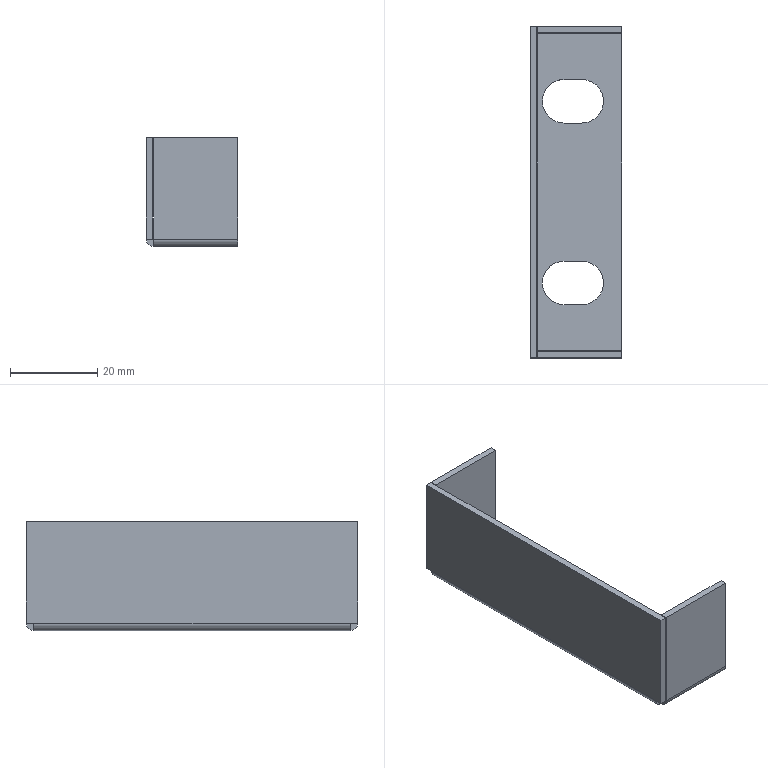Part | SolidWorks | features Cut 5, EdgeFlange 3, ICE 2, FlatPattern 1, MirrorPattern 1, SMBaseFlange 1, SheetMetal 1 | 1 solid | 42 faces | box 21 x 76 x 25 mm | volume 6000 mm3 | plane 30 | cylinder 12 | commonest cylinder face diameters 10 x6 0.4 x3 3.4 x3
STEP:
#1=CARTESIAN_POINT('',(-2.7,25.8,0.));
#2=VERTEX_POINT('',#1);
#3=CARTESIAN_POINT('',(-7.7,20.8,0.));
#4=VERTEX_POINT('',#3);
#5=CARTESIAN_POINT('',(-2.7,20.8,0.));
#6=DIRECTION('',(0.,0.,1.));
#7=DIRECTION('',(1.,0.,0.));
#8=AXIS2_PLACEMENT_3D('',#5,#6,#7);
#9=CIRCLE('',#8,5.);
#10=EDGE_CURVE('',#2,#4,#9,.T.);
#11=ORIENTED_EDGE('',*,*,#10,.T.);
#12=CARTESIAN_POINT('',(-7.7,20.8,-1.5));
#13=VERTEX_POINT('',#12);
#14=CARTESIAN_POINT('',(-7.7,20.8,8.5));
#15=DIRECTION('',(0.,0.,-1.));
#16=VECTOR('',#15,1000.);
#17=LINE('',#14,#16);
#18=EDGE_CURVE('',#4,#13,#17,.T.);
#19=ORIENTED_EDGE('',*,*,#18,.T.);
#20=CARTESIAN_POINT('',(-2.7,25.8,-1.5));
#21=VERTEX_POINT('',#20);
#22=CARTESIAN_POINT('',(-2.7,20.8,-1.5));
#23=DIRECTION('',(0.,0.,-1.));
#24=DIRECTION('',(-1.,0.,0.));
#25=AXIS2_PLACEMENT_3D('',#22,#23,#24);
#26=CIRCLE('',#25,5.);
#27=EDGE_CURVE('',#13,#21,#26,.T.);
#28=ORIENTED_EDGE('',*,*,#27,.T.);
#29=CARTESIAN_POINT('',(-2.7,25.8,8.5));
#30=DIRECTION('',(0.,0.,-1.));
#31=VECTOR('',#30,1000.);
#32=LINE('',#29,#31);
#33=EDGE_CURVE('',#2,#21,#32,.T.);
#34=ORIENTED_EDGE('',*,*,#33,.F.);
#35=EDGE_LOOP('',(#11,#19,#28,#34));
#36=FACE_OUTER_BOUND('',#35,.T.);
#37=CARTESIAN_POINT('',(-2.7,20.8,8.5));
#38=DIRECTION('',(0.,0.,-1.));
#39=DIRECTION('',(-1.,0.,0.));
#40=AXIS2_PLACEMENT_3D('',#37,#38,#39);
#41=CYLINDRICAL_SURFACE('',#40,5.);
#42=ADVANCED_FACE('',(#36),#41,.F.);
#43=CARTESIAN_POINT('',(-2.7,-15.8,0.));
#44=VERTEX_POINT('',#43);
#45=CARTESIAN_POINT('',(-7.7,-20.8,0.));
#46=VERTEX_POINT('',#45);
#47=CARTESIAN_POINT('',(-2.7,-20.8,0.));
#48=DIRECTION('',(0.,0.,1.));
#49=DIRECTION('',(1.,0.,0.));
#50=AXIS2_PLACEMENT_3D('',#47,#48,#49);
#51=CIRCLE('',#50,5.);
#52=EDGE_CURVE('',#44,#46,#51,.T.);
#53=ORIENTED_EDGE('',*,*,#52,.T.);
#54=CARTESIAN_POINT('',(-7.7,-20.8,-1.5));
#55=VERTEX_POINT('',#54);
#56=CARTESIAN_POINT('',(-7.7,-20.8,8.5));
#57=DIRECTION('',(0.,0.,-1.));
#58=VECTOR('',#57,1000.);
#59=LINE('',#56,#58);
#60=EDGE_CURVE('',#46,#55,#59,.T.);
#61=ORIENTED_EDGE('',*,*,#60,.T.);
#62=CARTESIAN_POINT('',(-2.7,-15.8,-1.5));
#63=VERTEX_POINT('',#62);
#64=CARTESIAN_POINT('',(-2.7,-20.8,-1.5));
#65=DIRECTION('',(0.,0.,-1.));
#66=DIRECTION('',(1.,0.,0.));
#67=AXIS2_PLACEMENT_3D('',#64,#65,#66);
#68=CIRCLE('',#67,5.);
#69=EDGE_CURVE('',#55,#63,#68,.T.);
#70=ORIENTED_EDGE('',*,*,#69,.T.);
#71=CARTESIAN_POINT('',(-2.7,-15.8,8.5));
#72=DIRECTION('',(0.,0.,-1.));
#73=VECTOR('',#72,1000.);
#74=LINE('',#71,#73);
#75=EDGE_CURVE('',#44,#63,#74,.T.);
#76=ORIENTED_EDGE('',*,*,#75,.F.);
#77=EDGE_LOOP('',(#53,#61,#70,#76));
#78=FACE_OUTER_BOUND('',#77,.T.);
#79=CARTESIAN_POINT('',(-2.7,-20.8,8.5));
#80=DIRECTION('',(0.,0.,-1.));
#81=DIRECTION('',(-1.,0.,0.));
#82=AXIS2_PLACEMENT_3D('',#79,#80,#81);
#83=CYLINDRICAL_SURFACE('',#82,5.);
#84=ADVANCED_FACE('',(#78),#83,.F.);
#85=CARTESIAN_POINT('',(-9.,-36.3,0.2));
#86=VERTEX_POINT('',#85);
#87=CARTESIAN_POINT('',(-10.5,-36.3,0.2));
#88=VERTEX_POINT('',#87);
#89=CARTESIAN_POINT('',(-9.,-36.3,0.2));
#90=DIRECTION('',(-1.,0.,0.));
#91=VECTOR('',#90,1000.);
#92=LINE('',#89,#91);
#93=EDGE_CURVE('',#86,#88,#92,.T.);
#94=ORIENTED_EDGE('',*,*,#93,.F.);
#95=CARTESIAN_POINT('',(-9.,-38.,0.2));
#96=VERTEX_POINT('',#95);
#97=CARTESIAN_POINT('',(-9.,38.,0.2));
#98=DIRECTION('',(0.,-1.,0.));
#99=VECTOR('',#98,1000.);
#100=LINE('',#97,#99);
#101=EDGE_CURVE('',#86,#96,#100,.T.);
#102=ORIENTED_EDGE('',*,*,#101,.T.);
#103=CARTESIAN_POINT('',(-10.5,-38.,0.2));
#104=VERTEX_POINT('',#103);
#105=CARTESIAN_POINT('',(-9.,-38.,0.2));
#106=DIRECTION('',(-1.,0.,0.));
#107=VECTOR('',#106,1000.);
#108=LINE('',#105,#107);
#109=EDGE_CURVE('',#96,#104,#108,.T.);
#110=ORIENTED_EDGE('',*,*,#109,.T.);
#111=CARTESIAN_POINT('',(-10.5,38.,0.2));
#112=DIRECTION('',(0.,1.,0.));
#113=VECTOR('',#112,1000.);
#114=LINE('',#111,#113);
#115=EDGE_CURVE('',#104,#88,#114,.T.);
#116=ORIENTED_EDGE('',*,*,#115,.T.);
#117=EDGE_LOOP('',(#94,#102,#110,#116));
#118=FACE_OUTER_BOUND('',#117,.T.);
#119=CARTESIAN_POINT('',(0.,0.,0.2));
#120=DIRECTION('',(0.,0.,1.));
#121=DIRECTION('',(1.,0.,0.));
#122=AXIS2_PLACEMENT_3D('',#119,#120,#121);
#123=PLANE('',#122);
#124=ADVANCED_FACE('',(#118),#123,.F.);
#125=CARTESIAN_POINT('',(-8.8,-36.3,-1.5));
#126=VERTEX_POINT('',#125);
#127=CARTESIAN_POINT('',(-8.8,36.3,-1.5));
#128=VERTEX_POINT('',#127);
#129=CARTESIAN_POINT('',(-8.8,-38.,-1.5));
#130=DIRECTION('',(0.,1.,0.));
#131=VECTOR('',#130,1000.);
#132=LINE('',#129,#131);
#133=EDGE_CURVE('',#126,#128,#132,.T.);
#134=ORIENTED_EDGE('',*,*,#133,.F.);
#135=CARTESIAN_POINT('',(-8.8,-36.3,0.2));
#136=DIRECTION('',(0.,1.,0.));
#137=DIRECTION('',(0.,0.,-1.));
#138=AXIS2_PLACEMENT_3D('',#135,#136,#137);
#139=CIRCLE('',#138,1.7);
#140=EDGE_CURVE('',#126,#88,#139,.T.);
#141=ORIENTED_EDGE('',*,*,#140,.T.);
#142=CARTESIAN_POINT('',(-10.5,36.3,0.2));
#143=VERTEX_POINT('',#142);
#144=CARTESIAN_POINT('',(-10.5,38.,0.2));
#145=DIRECTION('',(0.,1.,0.));
#146=VECTOR('',#145,1000.);
#147=LINE('',#144,#146);
#148=EDGE_CURVE('',#88,#143,#147,.T.);
#149=ORIENTED_EDGE('',*,*,#148,.T.);
#150=CARTESIAN_POINT('',(-8.8,36.3,0.2));
#151=DIRECTION('',(0.,-1.,0.));
#152=DIRECTION('',(0.,0.,1.));
#153=AXIS2_PLACEMENT_3D('',#150,#151,#152);
#154=CIRCLE('',#153,1.7);
#155=EDGE_CURVE('',#143,#128,#154,.T.);
#156=ORIENTED_EDGE('',*,*,#155,.T.);
#157=EDGE_LOOP('',(#134,#141,#149,#156));
#158=FACE_OUTER_BOUND('',#157,.T.);
#159=CARTESIAN_POINT('',(-8.8,-38.,0.2));
#160=DIRECTION('',(0.,-1.,0.));
#161=DIRECTION('',(-1.,0.,0.));
#162=AXIS2_PLACEMENT_3D('',#159,#160,#161);
#163=CYLINDRICAL_SURFACE('',#162,1.7);
#164=ADVANCED_FACE('',(#158),#163,.T.);
#165=CARTESIAN_POINT('',(-8.8,-36.3,0.));
#166=VERTEX_POINT('',#165);
#167=CARTESIAN_POINT('',(-8.8,-36.3,0.2));
#168=DIRECTION('',(0.,1.,0.));
#169=DIRECTION('',(0.,0.,-1.));
#170=AXIS2_PLACEMENT_3D('',#167,#168,#169);
#171=CIRCLE('',#170,0.2);
#172=EDGE_CURVE('',#166,#86,#171,.T.);
#173=ORIENTED_EDGE('',*,*,#172,.T.);
#174=ORIENTED_EDGE('',*,*,#93,.T.);
#175=ORIENTED_EDGE('',*,*,#140,.F.);
#176=CARTESIAN_POINT('',(-8.8,-36.3,0.));
#177=DIRECTION('',(0.,0.,-1.));
#178=VECTOR('',#177,1000.);
#179=LINE('',#176,#178);
#180=EDGE_CURVE('',#166,#126,#179,.T.);
#181=ORIENTED_EDGE('',*,*,#180,.F.);
#182=EDGE_LOOP('',(#173,#174,#175,#181));
#183=FACE_OUTER_BOUND('',#182,.T.);
#184=CARTESIAN_POINT('',(-8.8,-36.3,0.2));
#185=DIRECTION('',(0.,-1.,0.));
#186=DIRECTION('',(0.,0.,-1.));
#187=AXIS2_PLACEMENT_3D('',#184,#185,#186);
#188=PLANE('',#187);
#189=ADVANCED_FACE('',(#183),#188,.T.);
#190=CARTESIAN_POINT('',(1.3,15.8,-1.5));
#191=VERTEX_POINT('',#190);
#192=CARTESIAN_POINT('',(-2.7,15.8,-1.5));
#193=VERTEX_POINT('',#192);
#194=CARTESIAN_POINT('',(1.3,15.8,-1.5));
#195=DIRECTION('',(-1.,0.,0.));
#196=VECTOR('',#195,1000.);
#197=LINE('',#194,#196);
#198=EDGE_CURVE('',#191,#193,#197,.T.);
#199=ORIENTED_EDGE('',*,*,#198,.F.);
#200=CARTESIAN_POINT('',(1.3,25.8,-1.5));
#201=VERTEX_POINT('',#200);
#202=CARTESIAN_POINT('',(1.3,20.8,-1.5));
#203=DIRECTION('',(0.,0.,-1.));
#204=DIRECTION('',(-1.,0.,0.));
#205=AXIS2_PLACEMENT_3D('',#202,#203,#204);
#206=CIRCLE('',#205,5.);
#207=EDGE_CURVE('',#201,#191,#206,.T.);
#208=ORIENTED_EDGE('',*,*,#207,.F.);
#209=CARTESIAN_POINT('',(1.3,25.8,-1.5));
#210=DIRECTION('',(1.,0.,0.));
#211=VECTOR('',#210,1000.);
#212=LINE('',#209,#211);
#213=EDGE_CURVE('',#21,#201,#212,.T.);
#214=ORIENTED_EDGE('',*,*,#213,.F.);
#215=ORIENTED_EDGE('',*,*,#27,.F.);
#216=CARTESIAN_POINT('',(-2.7,20.8,-1.5));
#217=DIRECTION('',(0.,0.,-1.));
#218=DIRECTION('',(-1.,0.,0.));
#219=AXIS2_PLACEMENT_3D('',#216,#217,#218);
#220=CIRCLE('',#219,5.);
#221=EDGE_CURVE('',#193,#13,#220,.T.);
#222=ORIENTED_EDGE('',*,*,#221,.F.);
#223=EDGE_LOOP('',(#199,#208,#214,#215,#222));
#224=FACE_BOUND('',#223,.T.);
#225=CARTESIAN_POINT('',(1.3,-25.8,-1.5));
#226=VERTEX_POINT('',#225);
#227=CARTESIAN_POINT('',(-2.7,-25.8,-1.5));
#228=VERTEX_POINT('',#227);
#229=CARTESIAN_POINT('',(1.3,-25.8,-1.5));
#230=DIRECTION('',(-1.,0.,0.));
#231=VECTOR('',#230,1000.);
#232=LINE('',#229,#231);
#233=EDGE_CURVE('',#226,#228,#232,.T.);
#234=ORIENTED_EDGE('',*,*,#233,.F.);
#235=CARTESIAN_POINT('',(1.3,-15.8,-1.5));
#236=VERTEX_POINT('',#235);
#237=CARTESIAN_POINT('',(1.3,-20.8,-1.5));
#238=DIRECTION('',(0.,0.,-1.));
#239=DIRECTION('',(1.,0.,0.));
#240=AXIS2_PLACEMENT_3D('',#237,#238,#239);
#241=CIRCLE('',#240,5.);
#242=EDGE_CURVE('',#236,#226,#241,.T.);
#243=ORIENTED_EDGE('',*,*,#242,.F.);
#244=CARTESIAN_POINT('',(1.3,-15.8,-1.5));
#245=DIRECTION('',(1.,0.,0.));
#246=VECTOR('',#245,1000.);
#247=LINE('',#244,#246);
#248=EDGE_CURVE('',#63,#236,#247,.T.);
#249=ORIENTED_EDGE('',*,*,#248,.F.);
#250=ORIENTED_EDGE('',*,*,#69,.F.);
#251=CARTESIAN_POINT('',(-2.7,-20.8,-1.5));
#252=DIRECTION('',(0.,0.,-1.));
#253=DIRECTION('',(1.,0.,0.));
#254=AXIS2_PLACEMENT_3D('',#251,#252,#253);
#255=CIRCLE('',#254,5.);
#256=EDGE_CURVE('',#228,#55,#255,.T.);
#257=ORIENTED_EDGE('',*,*,#256,.F.);
#258=EDGE_LOOP('',(#234,#243,#249,#250,#257));
#259=FACE_BOUND('',#258,.T.);
#260=CARTESIAN_POINT('',(10.5,-36.3,-1.5));
#261=VERTEX_POINT('',#260);
#262=CARTESIAN_POINT('',(10.5,-36.3,-1.5));
#263=DIRECTION('',(-1.,0.,0.));
#264=VECTOR('',#263,1000.);
#265=LINE('',#262,#264);
#266=EDGE_CURVE('',#261,#126,#265,.T.);
#267=ORIENTED_EDGE('',*,*,#266,.T.);
#268=ORIENTED_EDGE('',*,*,#133,.T.);
#269=CARTESIAN_POINT('',(10.5,36.3,-1.5));
#270=VERTEX_POINT('',#269);
#271=CARTESIAN_POINT('',(-8.8,36.3,-1.5));
#272=DIRECTION('',(1.,0.,0.));
#273=VECTOR('',#272,1000.);
#274=LINE('',#271,#273);
#275=EDGE_CURVE('',#128,#270,#274,.T.);
#276=ORIENTED_EDGE('',*,*,#275,.T.);
#277=CARTESIAN_POINT('',(10.5,38.,-1.5));
#278=DIRECTION('',(0.,1.,0.));
#279=VECTOR('',#278,1000.);
#280=LINE('',#277,#279);
#281=EDGE_CURVE('',#261,#270,#280,.T.);
#282=ORIENTED_EDGE('',*,*,#281,.F.);
#283=EDGE_LOOP('',(#267,#268,#276,#282));
#284=FACE_OUTER_BOUND('',#283,.T.);
#285=CARTESIAN_POINT('',(0.,0.,-1.5));
#286=DIRECTION('',(0.,0.,1.));
#287=DIRECTION('',(1.,0.,0.));
#288=AXIS2_PLACEMENT_3D('',#285,#286,#287);
#289=PLANE('',#288);
#290=ADVANCED_FACE('',(#224,#259,#284),#289,.F.);
#291=CARTESIAN_POINT('',(1.3,15.8,0.));
#292=VERTEX_POINT('',#291);
#293=CARTESIAN_POINT('',(1.3,25.8,0.));
#294=VERTEX_POINT('',#293);
#295=CARTESIAN_POINT('',(1.3,20.8,0.));
#296=DIRECTION('',(0.,0.,1.));
#297=DIRECTION('',(1.,0.,0.));
#298=AXIS2_PLACEMENT_3D('',#295,#296,#297);
#299=CIRCLE('',#298,5.);
#300=EDGE_CURVE('',#292,#294,#299,.T.);
#301=ORIENTED_EDGE('',*,*,#300,.F.);
#302=CARTESIAN_POINT('',(-2.7,15.8,0.));
#303=VERTEX_POINT('',#302);
#304=CARTESIAN_POINT('',(0.,15.8,0.));
#305=DIRECTION('',(1.,0.,0.));
#306=VECTOR('',#305,1000.);
#307=LINE('',#304,#306);
#308=EDGE_CURVE('',#303,#292,#307,.T.);
#309=ORIENTED_EDGE('',*,*,#308,.F.);
#310=CARTESIAN_POINT('',(-2.7,20.8,0.));
#311=DIRECTION('',(0.,0.,1.));
#312=DIRECTION('',(1.,0.,0.));
#313=AXIS2_PLACEMENT_3D('',#310,#311,#312);
#314=CIRCLE('',#313,5.);
#315=EDGE_CURVE('',#4,#303,#314,.T.);
#316=ORIENTED_EDGE('',*,*,#315,.F.);
#317=ORIENTED_EDGE('',*,*,#10,.F.);
#318=CARTESIAN_POINT('',(0.,25.8,0.));
#319=DIRECTION('',(-1.,0.,0.));
#320=VECTOR('',#319,1000.);
#321=LINE('',#318,#320);
#322=EDGE_CURVE('',#294,#2,#321,.T.);
#323=ORIENTED_EDGE('',*,*,#322,.F.);
#324=EDGE_LOOP('',(#301,#309,#316,#317,#323));
#325=FACE_BOUND('',#324,.T.);
#326=CARTESIAN_POINT('',(1.3,-25.8,0.));
#327=VERTEX_POINT('',#326);
#328=CARTESIAN_POINT('',(1.3,-15.8,0.));
#329=VERTEX_POINT('',#328);
#330=CARTESIAN_POINT('',(1.3,-20.8,0.));
#331=DIRECTION('',(0.,0.,1.));
#332=DIRECTION('',(1.,0.,0.));
#333=AXIS2_PLACEMENT_3D('',#330,#331,#332);
#334=CIRCLE('',#333,5.);
#335=EDGE_CURVE('',#327,#329,#334,.T.);
#336=ORIENTED_EDGE('',*,*,#335,.F.);
#337=CARTESIAN_POINT('',(-2.7,-25.8,0.));
#338=VERTEX_POINT('',#337);
#339=CARTESIAN_POINT('',(0.,-25.8,0.));
#340=DIRECTION('',(1.,0.,0.));
#341=VECTOR('',#340,1000.);
#342=LINE('',#339,#341);
#343=EDGE_CURVE('',#338,#327,#342,.T.);
#344=ORIENTED_EDGE('',*,*,#343,.F.);
#345=CARTESIAN_POINT('',(-2.7,-20.8,0.));
#346=DIRECTION('',(0.,0.,1.));
#347=DIRECTION('',(1.,0.,0.));
#348=AXIS2_PLACEMENT_3D('',#345,#346,#347);
#349=CIRCLE('',#348,5.);
#350=EDGE_CURVE('',#46,#338,#349,.T.);
#351=ORIENTED_EDGE('',*,*,#350,.F.);
#352=ORIENTED_EDGE('',*,*,#52,.F.);
#353=CARTESIAN_POINT('',(0.,-15.8,0.));
#354=DIRECTION('',(-1.,0.,0.));
#355=VECTOR('',#354,1000.);
#356=LINE('',#353,#355);
#357=EDGE_CURVE('',#329,#44,#356,.T.);
#358=ORIENTED_EDGE('',*,*,#357,.F.);
#359=EDGE_LOOP('',(#336,#344,#351,#352,#358));
#360=FACE_BOUND('',#359,.T.);
#361=CARTESIAN_POINT('',(-8.8,36.3,0.));
#362=VERTEX_POINT('',#361);
#363=CARTESIAN_POINT('',(-8.8,-38.,0.));
#364=DIRECTION('',(0.,1.,0.));
#365=VECTOR('',#364,1000.);
#366=LINE('',#363,#365);
#367=EDGE_CURVE('',#166,#362,#366,.T.);
#368=ORIENTED_EDGE('',*,*,#367,.F.);
#369=CARTESIAN_POINT('',(10.5,-36.3,0.));
#370=VERTEX_POINT('',#369);
#371=CARTESIAN_POINT('',(10.5,-36.3,0.));
#372=DIRECTION('',(-1.,0.,0.));
#373=VECTOR('',#372,1000.);
#374=LINE('',#371,#373);
#375=EDGE_CURVE('',#370,#166,#374,.T.);
#376=ORIENTED_EDGE('',*,*,#375,.F.);
#377=CARTESIAN_POINT('',(10.5,36.3,0.));
#378=VERTEX_POINT('',#377);
#379=CARTESIAN_POINT('',(10.5,38.,0.));
#380=DIRECTION('',(0.,1.,0.));
#381=VECTOR('',#380,1000.);
#382=LINE('',#379,#381);
#383=EDGE_CURVE('',#370,#378,#382,.T.);
#384=ORIENTED_EDGE('',*,*,#383,.T.);
#385=CARTESIAN_POINT('',(-8.8,36.3,0.));
#386=DIRECTION('',(1.,0.,0.));
#387=VECTOR('',#386,1000.);
#388=LINE('',#385,#387);
#389=EDGE_CURVE('',#362,#378,#388,.T.);
#390=ORIENTED_EDGE('',*,*,#389,.F.);
#391=EDGE_LOOP('',(#368,#376,#384,#390));
#392=FACE_OUTER_BOUND('',#391,.T.);
#393=CARTESIAN_POINT('',(0.,0.,0.));
#394=DIRECTION('',(0.,0.,1.));
#395=DIRECTION('',(1.,0.,0.));
#396=AXIS2_PLACEMENT_3D('',#393,#394,#395);
#397=PLANE('',#396);
#398=ADVANCED_FACE('',(#325,#360,#392),#397,.T.);
#399=ORIENTED_EDGE('',*,*,#383,.F.);
#400=CARTESIAN_POINT('',(10.5,-36.3,0.));
#401=DIRECTION('',(0.,0.,-1.));
#402=VECTOR('',#401,1000.);
#403=LINE('',#400,#402);
#404=EDGE_CURVE('',#370,#261,#403,.T.);
#405=ORIENTED_EDGE('',*,*,#404,.T.);
#406=ORIENTED_EDGE('',*,*,#281,.T.);
#407=CARTESIAN_POINT('',(10.5,36.3,0.));
#408=DIRECTION('',(0.,0.,-1.));
#409=VECTOR('',#408,1000.);
#410=LINE('',#407,#409);
#411=EDGE_CURVE('',#378,#270,#410,.T.);
#412=ORIENTED_EDGE('',*,*,#411,.F.);
#413=EDGE_LOOP('',(#399,#405,#406,#412));
#414=FACE_OUTER_BOUND('',#413,.T.);
#415=CARTESIAN_POINT('',(10.5,38.,-1.5));
#416=DIRECTION('',(1.,0.,0.));
#417=DIRECTION('',(0.,0.,-1.));
#418=AXIS2_PLACEMENT_3D('',#415,#416,#417);
#419=PLANE('',#418);
#420=ADVANCED_FACE('',(#414),#419,.T.);
#421=CARTESIAN_POINT('',(-9.,36.3,0.2));
#422=VERTEX_POINT('',#421);
#423=CARTESIAN_POINT('',(-10.5,36.3,0.2));
#424=DIRECTION('',(1.,0.,0.));
#425=VECTOR('',#424,1000.);
#426=LINE('',#423,#425);
#427=EDGE_CURVE('',#143,#422,#426,.T.);
#428=ORIENTED_EDGE('',*,*,#427,.F.);
#429=CARTESIAN_POINT('',(-10.5,38.,0.2));
#430=VERTEX_POINT('',#429);
#431=CARTESIAN_POINT('',(-10.5,38.,0.2));
#432=DIRECTION('',(0.,1.,0.));
#433=VECTOR('',#432,1000.);
#434=LINE('',#431,#433);
#435=EDGE_CURVE('',#143,#430,#434,.T.);
#436=ORIENTED_EDGE('',*,*,#435,.T.);
#437=CARTESIAN_POINT('',(-9.,38.,0.2));
#438=VERTEX_POINT('',#437);
#439=CARTESIAN_POINT('',(-10.5,38.,0.2));
#440=DIRECTION('',(-1.,0.,0.));
#441=VECTOR('',#440,1000.);
#442=LINE('',#439,#441);
#443=EDGE_CURVE('',#438,#430,#442,.T.);
#444=ORIENTED_EDGE('',*,*,#443,.F.);
#445=CARTESIAN_POINT('',(-9.,38.,0.2));
#446=DIRECTION('',(0.,-1.,0.));
#447=VECTOR('',#446,1000.);
#448=LINE('',#445,#447);
#449=EDGE_CURVE('',#438,#422,#448,.T.);
#450=ORIENTED_EDGE('',*,*,#449,.T.);
#451=EDGE_LOOP('',(#428,#436,#444,#450));
#452=FACE_OUTER_BOUND('',#451,.T.);
#453=CARTESIAN_POINT('',(0.,0.,0.2));
#454=DIRECTION('',(0.,0.,-1.));
#455=DIRECTION('',(-1.,0.,0.));
#456=AXIS2_PLACEMENT_3D('',#453,#454,#455);
#457=PLANE('',#456);
#458=ADVANCED_FACE('',(#452),#457,.T.);
#459=ORIENTED_EDGE('',*,*,#155,.F.);
#460=ORIENTED_EDGE('',*,*,#427,.T.);
#461=CARTESIAN_POINT('',(-8.8,36.3,0.2));
#462=DIRECTION('',(0.,-1.,0.));
#463=DIRECTION('',(0.,0.,1.));
#464=AXIS2_PLACEMENT_3D('',#461,#462,#463);
#465=CIRCLE('',#464,0.2);
#466=EDGE_CURVE('',#422,#362,#465,.T.);
#467=ORIENTED_EDGE('',*,*,#466,.T.);
#468=CARTESIAN_POINT('',(-8.8,36.3,0.));
#469=DIRECTION('',(0.,0.,-1.));
#470=VECTOR('',#469,1000.);
#471=LINE('',#468,#470);
#472=EDGE_CURVE('',#362,#128,#471,.T.);
#473=ORIENTED_EDGE('',*,*,#472,.T.);
#474=EDGE_LOOP('',(#459,#460,#467,#473));
#475=FACE_OUTER_BOUND('',#474,.T.);
#476=CARTESIAN_POINT('',(-8.8,36.3,0.2));
#477=DIRECTION('',(0.,1.,0.));
#478=DIRECTION('',(0.,0.,1.));
#479=AXIS2_PLACEMENT_3D('',#476,#477,#478);
#480=PLANE('',#479);
#481=ADVANCED_FACE('',(#475),#480,.T.);
#482=ORIENTED_EDGE('',*,*,#172,.F.);
#483=ORIENTED_EDGE('',*,*,#367,.T.);
#484=ORIENTED_EDGE('',*,*,#466,.F.);
#485=CARTESIAN_POINT('',(-9.,38.,0.2));
#486=DIRECTION('',(0.,-1.,0.));
#487=VECTOR('',#486,1000.);
#488=LINE('',#485,#487);
#489=EDGE_CURVE('',#422,#86,#488,.T.);
#490=ORIENTED_EDGE('',*,*,#489,.T.);
#491=EDGE_LOOP('',(#482,#483,#484,#490));
#492=FACE_OUTER_BOUND('',#491,.T.);
#493=CARTESIAN_POINT('',(-8.8,-38.,0.2));
#494=DIRECTION('',(0.,-1.,0.));
#495=DIRECTION('',(-1.,0.,0.));
#496=AXIS2_PLACEMENT_3D('',#493,#494,#495);
#497=CYLINDRICAL_SURFACE('',#496,0.2);
#498=ADVANCED_FACE('',(#492),#497,.F.);
#499=ORIENTED_EDGE('',*,*,#443,.T.);
#500=CARTESIAN_POINT('',(-10.5,38.,23.5));
#501=VERTEX_POINT('',#500);
#502=CARTESIAN_POINT('',(-10.5,38.,0.));
#503=DIRECTION('',(0.,0.,-1.));
#504=VECTOR('',#503,1000.);
#505=LINE('',#502,#504);
#506=EDGE_CURVE('',#501,#430,#505,.T.);
#507=ORIENTED_EDGE('',*,*,#506,.F.);
#508=CARTESIAN_POINT('',(-9.,38.,23.5));
#509=VERTEX_POINT('',#508);
#510=CARTESIAN_POINT('',(-10.5,38.,23.5));
#511=DIRECTION('',(1.,0.,0.));
#512=VECTOR('',#511,1000.);
#513=LINE('',#510,#512);
#514=EDGE_CURVE('',#501,#509,#513,.T.);
#515=ORIENTED_EDGE('',*,*,#514,.T.);
#516=CARTESIAN_POINT('',(-9.,38.,0.));
#517=DIRECTION('',(0.,0.,-1.));
#518=VECTOR('',#517,1000.);
#519=LINE('',#516,#518);
#520=EDGE_CURVE('',#509,#438,#519,.T.);
#521=ORIENTED_EDGE('',*,*,#520,.T.);
#522=EDGE_LOOP('',(#499,#507,#515,#521));
#523=FACE_OUTER_BOUND('',#522,.T.);
#524=CARTESIAN_POINT('',(-10.5,38.,0.));
#525=DIRECTION('',(0.,-1.,0.));
#526=DIRECTION('',(0.,0.,-1.));
#527=AXIS2_PLACEMENT_3D('',#524,#525,#526);
#528=PLANE('',#527);
#529=ADVANCED_FACE('',(#523),#528,.F.);
#530=ORIENTED_EDGE('',*,*,#109,.F.);
#531=CARTESIAN_POINT('',(-9.,-38.,23.5));
#532=VERTEX_POINT('',#531);
#533=CARTESIAN_POINT('',(-9.,-38.,23.5));
#534=DIRECTION('',(0.,0.,1.));
#535=VECTOR('',#534,1000.);
#536=LINE('',#533,#535);
#537=EDGE_CURVE('',#96,#532,#536,.T.);
#538=ORIENTED_EDGE('',*,*,#537,.T.);
#539=CARTESIAN_POINT('',(-10.5,-38.,23.5));
#540=VERTEX_POINT('',#539);
#541=CARTESIAN_POINT('',(-10.5,-38.,23.5));
#542=DIRECTION('',(1.,0.,0.));
#543=VECTOR('',#542,1000.);
#544=LINE('',#541,#543);
#545=EDGE_CURVE('',#540,#532,#544,.T.);
#546=ORIENTED_EDGE('',*,*,#545,.F.);
#547=CARTESIAN_POINT('',(-10.5,-38.,0.));
#548=DIRECTION('',(0.,0.,1.));
#549=VECTOR('',#548,1000.);
#550=LINE('',#547,#549);
#551=EDGE_CURVE('',#104,#540,#550,.T.);
#552=ORIENTED_EDGE('',*,*,#551,.F.);
#553=EDGE_LOOP('',(#530,#538,#546,#552));
#554=FACE_OUTER_BOUND('',#553,.T.);
#555=CARTESIAN_POINT('',(-10.5,-38.,23.5));
#556=DIRECTION('',(0.,1.,0.));
#557=DIRECTION('',(0.,0.,1.));
#558=AXIS2_PLACEMENT_3D('',#555,#556,#557);
#559=PLANE('',#558);
#560=ADVANCED_FACE('',(#554),#559,.F.);
#561=ORIENTED_EDGE('',*,*,#115,.F.);
#562=ORIENTED_EDGE('',*,*,#551,.T.);
#563=CARTESIAN_POINT('',(-10.5,0.,23.5));
#564=DIRECTION('',(0.,1.,0.));
#565=VECTOR('',#564,1000.);
#566=LINE('',#563,#565);
#567=EDGE_CURVE('',#540,#501,#566,.T.);
#568=ORIENTED_EDGE('',*,*,#567,.T.);
#569=ORIENTED_EDGE('',*,*,#506,.T.);
#570=ORIENTED_EDGE('',*,*,#435,.F.);
#571=ORIENTED_EDGE('',*,*,#148,.F.);
#572=EDGE_LOOP('',(#561,#562,#568,#569,#570,#571));
#573=FACE_OUTER_BOUND('',#572,.T.);
#574=CARTESIAN_POINT('',(-10.5,0.,0.));
#575=DIRECTION('',(1.,0.,0.));
#576=DIRECTION('',(0.,0.,-1.));
#577=AXIS2_PLACEMENT_3D('',#574,#575,#576);
#578=PLANE('',#577);
#579=ADVANCED_FACE('',(#573),#578,.F.);
#580=ORIENTED_EDGE('',*,*,#537,.F.);
#581=ORIENTED_EDGE('',*,*,#101,.F.);
#582=ORIENTED_EDGE('',*,*,#489,.F.);
#583=ORIENTED_EDGE('',*,*,#449,.F.);
#584=ORIENTED_EDGE('',*,*,#520,.F.);
#585=CARTESIAN_POINT('',(-9.,38.,23.5));
#586=DIRECTION('',(0.,1.,0.));
#587=VECTOR('',#586,1000.);
#588=LINE('',#585,#587);
#589=EDGE_CURVE('',#532,#509,#588,.T.);
#590=ORIENTED_EDGE('',*,*,#589,.F.);
#591=EDGE_LOOP('',(#580,#581,#582,#583,#584,#590));
#592=FACE_OUTER_BOUND('',#591,.T.);
#593=CARTESIAN_POINT('',(-9.,0.,0.));
#594=DIRECTION('',(1.,0.,0.));
#595=DIRECTION('',(0.,0.,-1.));
#596=AXIS2_PLACEMENT_3D('',#593,#594,#595);
#597=PLANE('',#596);
#598=ADVANCED_FACE('',(#592),#597,.T.);
#599=ORIENTED_EDGE('',*,*,#589,.T.);
#600=ORIENTED_EDGE('',*,*,#514,.F.);
#601=ORIENTED_EDGE('',*,*,#567,.F.);
#602=ORIENTED_EDGE('',*,*,#545,.T.);
#603=EDGE_LOOP('',(#599,#600,#601,#602));
#604=FACE_OUTER_BOUND('',#603,.T.);
#605=CARTESIAN_POINT('',(-10.5,38.,23.5));
#606=DIRECTION('',(0.,0.,-1.));
#607=DIRECTION('',(-1.,0.,0.));
#608=AXIS2_PLACEMENT_3D('',#605,#606,#607);
#609=PLANE('',#608);
#610=ADVANCED_FACE('',(#604),#609,.F.);
#611=CARTESIAN_POINT('',(10.5,36.5,0.2));
#612=VERTEX_POINT('',#611);
#613=CARTESIAN_POINT('',(10.5,38.,0.2));
#614=VERTEX_POINT('',#613);
#615=CARTESIAN_POINT('',(10.5,38.,0.2));
#616=DIRECTION('',(0.,1.,0.));
#617=VECTOR('',#616,1000.);
#618=LINE('',#615,#617);
#619=EDGE_CURVE('',#612,#614,#618,.T.);
#620=ORIENTED_EDGE('',*,*,#619,.F.);
#621=CARTESIAN_POINT('',(10.5,36.3,0.2));
#622=DIRECTION('',(1.,0.,0.));
#623=DIRECTION('',(0.,0.,1.));
#624=AXIS2_PLACEMENT_3D('',#621,#622,#623);
#625=CIRCLE('',#624,0.2);
#626=EDGE_CURVE('',#378,#612,#625,.T.);
#627=ORIENTED_EDGE('',*,*,#626,.F.);
#628=ORIENTED_EDGE('',*,*,#411,.T.);
#629=CARTESIAN_POINT('',(10.5,36.3,0.2));
#630=DIRECTION('',(1.,0.,0.));
#631=DIRECTION('',(0.,0.,1.));
#632=AXIS2_PLACEMENT_3D('',#629,#630,#631);
#633=CIRCLE('',#632,1.7);
#634=EDGE_CURVE('',#270,#614,#633,.T.);
#635=ORIENTED_EDGE('',*,*,#634,.T.);
#636=EDGE_LOOP('',(#620,#627,#628,#635));
#637=FACE_OUTER_BOUND('',#636,.T.);
#638=CARTESIAN_POINT('',(10.5,36.3,0.2));
#639=DIRECTION('',(1.,0.,0.));
#640=DIRECTION('',(0.,0.,-1.));
#641=AXIS2_PLACEMENT_3D('',#638,#639,#640);
#642=PLANE('',#641);
#643=ADVANCED_FACE('',(#637),#642,.T.);
#644=CARTESIAN_POINT('',(-8.8,36.5,0.2));
#645=VERTEX_POINT('',#644);
#646=CARTESIAN_POINT('',(-8.8,36.3,0.2));
#647=DIRECTION('',(-1.,0.,0.));
#648=DIRECTION('',(0.,0.,1.));
#649=AXIS2_PLACEMENT_3D('',#646,#647,#648);
#650=CIRCLE('',#649,0.2);
#651=EDGE_CURVE('',#645,#362,#650,.T.);
#652=ORIENTED_EDGE('',*,*,#651,.F.);
#653=CARTESIAN_POINT('',(-8.8,38.,0.2));
#654=VERTEX_POINT('',#653);
#655=CARTESIAN_POINT('',(-8.8,36.5,0.2));
#656=DIRECTION('',(0.,1.,0.));
#657=VECTOR('',#656,1000.);
#658=LINE('',#655,#657);
#659=EDGE_CURVE('',#645,#654,#658,.T.);
#660=ORIENTED_EDGE('',*,*,#659,.T.);
#661=CARTESIAN_POINT('',(-8.8,36.3,0.2));
#662=DIRECTION('',(-1.,0.,0.));
#663=DIRECTION('',(0.,0.,1.));
#664=AXIS2_PLACEMENT_3D('',#661,#662,#663);
#665=CIRCLE('',#664,1.7);
#666=EDGE_CURVE('',#654,#128,#665,.T.);
#667=ORIENTED_EDGE('',*,*,#666,.T.);
#668=ORIENTED_EDGE('',*,*,#472,.F.);
#669=EDGE_LOOP('',(#652,#660,#667,#668));
#670=FACE_OUTER_BOUND('',#669,.T.);
#671=CARTESIAN_POINT('',(-8.8,36.3,0.2));
#672=DIRECTION('',(1.,0.,0.));
#673=DIRECTION('',(0.,0.,-1.));
#674=AXIS2_PLACEMENT_3D('',#671,#672,#673);
#675=PLANE('',#674);
#676=ADVANCED_FACE('',(#670),#675,.F.);
#677=ORIENTED_EDGE('',*,*,#275,.F.);
#678=ORIENTED_EDGE('',*,*,#666,.F.);
#679=CARTESIAN_POINT('',(10.5,38.,0.2));
#680=DIRECTION('',(1.,0.,0.));
#681=VECTOR('',#680,1000.);
#682=LINE('',#679,#681);
#683=EDGE_CURVE('',#654,#614,#682,.T.);
#684=ORIENTED_EDGE('',*,*,#683,.T.);
#685=ORIENTED_EDGE('',*,*,#634,.F.);
#686=EDGE_LOOP('',(#677,#678,#684,#685));
#687=FACE_OUTER_BOUND('',#686,.T.);
#688=CARTESIAN_POINT('',(-8.8,36.3,0.2));
#689=DIRECTION('',(-1.,0.,0.));
#690=DIRECTION('',(0.,1.,0.));
#691=AXIS2_PLACEMENT_3D('',#688,#689,#690);
#692=CYLINDRICAL_SURFACE('',#691,1.7);
#693=ADVANCED_FACE('',(#687),#692,.T.);
#694=ORIENTED_EDGE('',*,*,#389,.T.);
#695=ORIENTED_EDGE('',*,*,#626,.T.);
#696=CARTESIAN_POINT('',(10.5,36.5,0.2));
#697=DIRECTION('',(-1.,0.,0.));
#698=VECTOR('',#697,1000.);
#699=LINE('',#696,#698);
#700=EDGE_CURVE('',#612,#645,#699,.T.);
#701=ORIENTED_EDGE('',*,*,#700,.T.);
#702=ORIENTED_EDGE('',*,*,#651,.T.);
#703=EDGE_LOOP('',(#694,#695,#701,#702));
#704=FACE_OUTER_BOUND('',#703,.T.);
#705=CARTESIAN_POINT('',(-8.8,36.3,0.2));
#706=DIRECTION('',(-1.,0.,0.));
#707=DIRECTION('',(0.,1.,0.));
#708=AXIS2_PLACEMENT_3D('',#705,#706,#707);
#709=CYLINDRICAL_SURFACE('',#708,0.2);
#710=ADVANCED_FACE('',(#704),#709,.F.);
#711=ORIENTED_EDGE('',*,*,#619,.T.);
#712=CARTESIAN_POINT('',(10.5,38.,23.5));
#713=VERTEX_POINT('',#712);
#714=CARTESIAN_POINT('',(10.5,38.,0.));
#715=DIRECTION('',(0.,0.,-1.));
#716=VECTOR('',#715,1000.);
#717=LINE('',#714,#716);
#718=EDGE_CURVE('',#713,#614,#717,.T.);
#719=ORIENTED_EDGE('',*,*,#718,.F.);
#720=CARTESIAN_POINT('',(10.5,36.5,23.5));
#721=VERTEX_POINT('',#720);
#722=CARTESIAN_POINT('',(10.5,38.,23.5));
#723=DIRECTION('',(0.,-1.,0.));
#724=VECTOR('',#723,1000.);
#725=LINE('',#722,#724);
#726=EDGE_CURVE('',#713,#721,#725,.T.);
#727=ORIENTED_EDGE('',*,*,#726,.T.);
#728=CARTESIAN_POINT('',(10.5,36.5,0.));
#729=DIRECTION('',(0.,0.,-1.));
#730=VECTOR('',#729,1000.);
#731=LINE('',#728,#730);
#732=EDGE_CURVE('',#721,#612,#731,.T.);
#733=ORIENTED_EDGE('',*,*,#732,.T.);
#734=EDGE_LOOP('',(#711,#719,#727,#733));
#735=FACE_OUTER_BOUND('',#734,.T.);
#736=CARTESIAN_POINT('',(10.5,38.,0.));
#737=DIRECTION('',(-1.,0.,0.));
#738=DIRECTION('',(0.,0.,1.));
#739=AXIS2_PLACEMENT_3D('',#736,#737,#738);
#740=PLANE('',#739);
#741=ADVANCED_FACE('',(#735),#740,.F.);
#742=ORIENTED_EDGE('',*,*,#659,.F.);
#743=CARTESIAN_POINT('',(-8.8,36.5,23.5));
#744=VERTEX_POINT('',#743);
#745=CARTESIAN_POINT('',(-8.8,36.5,23.5));
#746=DIRECTION('',(0.,0.,1.));
#747=VECTOR('',#746,1000.);
#748=LINE('',#745,#747);
#749=EDGE_CURVE('',#645,#744,#748,.T.);
#750=ORIENTED_EDGE('',*,*,#749,.T.);
#751=CARTESIAN_POINT('',(-8.8,38.,23.5));
#752=VERTEX_POINT('',#751);
#753=CARTESIAN_POINT('',(-8.8,38.,23.5));
#754=DIRECTION('',(0.,-1.,0.));
#755=VECTOR('',#754,1000.);
#756=LINE('',#753,#755);
#757=EDGE_CURVE('',#752,#744,#756,.T.);
#758=ORIENTED_EDGE('',*,*,#757,.F.);
#759=CARTESIAN_POINT('',(-8.8,38.,0.));
#760=DIRECTION('',(0.,0.,1.));
#761=VECTOR('',#760,1000.);
#762=LINE('',#759,#761);
#763=EDGE_CURVE('',#654,#752,#762,.T.);
#764=ORIENTED_EDGE('',*,*,#763,.F.);
#765=EDGE_LOOP('',(#742,#750,#758,#764));
#766=FACE_OUTER_BOUND('',#765,.T.);
#767=CARTESIAN_POINT('',(-8.8,38.,23.5));
#768=DIRECTION('',(1.,0.,0.));
#769=DIRECTION('',(0.,0.,-1.));
#770=AXIS2_PLACEMENT_3D('',#767,#768,#769);
#771=PLANE('',#770);
#772=ADVANCED_FACE('',(#766),#771,.F.);
#773=ORIENTED_EDGE('',*,*,#683,.F.);
#774=ORIENTED_EDGE('',*,*,#763,.T.);
#775=CARTESIAN_POINT('',(0.,38.,23.5));
#776=DIRECTION('',(1.,0.,0.));
#777=VECTOR('',#776,1000.);
#778=LINE('',#775,#777);
#779=EDGE_CURVE('',#752,#713,#778,.T.);
#780=ORIENTED_EDGE('',*,*,#779,.T.);
#781=ORIENTED_EDGE('',*,*,#718,.T.);
#782=EDGE_LOOP('',(#773,#774,#780,#781));
#783=FACE_OUTER_BOUND('',#782,.T.);
#784=CARTESIAN_POINT('',(0.,38.,0.));
#785=DIRECTION('',(0.,-1.,0.));
#786=DIRECTION('',(0.,0.,-1.));
#787=AXIS2_PLACEMENT_3D('',#784,#785,#786);
#788=PLANE('',#787);
#789=ADVANCED_FACE('',(#783),#788,.F.);
#790=ORIENTED_EDGE('',*,*,#749,.F.);
#791=ORIENTED_EDGE('',*,*,#700,.F.);
#792=ORIENTED_EDGE('',*,*,#732,.F.);
#793=CARTESIAN_POINT('',(10.5,36.5,23.5));
#794=DIRECTION('',(1.,0.,0.));
#795=VECTOR('',#794,1000.);
#796=LINE('',#793,#795);
#797=EDGE_CURVE('',#744,#721,#796,.T.);
#798=ORIENTED_EDGE('',*,*,#797,.F.);
#799=EDGE_LOOP('',(#790,#791,#792,#798));
#800=FACE_OUTER_BOUND('',#799,.T.);
#801=CARTESIAN_POINT('',(0.,36.5,0.));
#802=DIRECTION('',(0.,-1.,0.));
#803=DIRECTION('',(0.,0.,-1.));
#804=AXIS2_PLACEMENT_3D('',#801,#802,#803);
#805=PLANE('',#804);
#806=ADVANCED_FACE('',(#800),#805,.T.);
#807=ORIENTED_EDGE('',*,*,#797,.T.);
#808=ORIENTED_EDGE('',*,*,#726,.F.);
#809=ORIENTED_EDGE('',*,*,#779,.F.);
#810=ORIENTED_EDGE('',*,*,#757,.T.);
#811=EDGE_LOOP('',(#807,#808,#809,#810));
#812=FACE_OUTER_BOUND('',#811,.T.);
#813=CARTESIAN_POINT('',(10.5,38.,23.5));
#814=DIRECTION('',(0.,0.,-1.));
#815=DIRECTION('',(0.,1.,0.));
#816=AXIS2_PLACEMENT_3D('',#813,#814,#815);
#817=PLANE('',#816);
#818=ADVANCED_FACE('',(#812),#817,.F.);
#819=CARTESIAN_POINT('',(-8.8,-36.5,0.2));
#820=VERTEX_POINT('',#819);
#821=CARTESIAN_POINT('',(-8.8,-38.,0.2));
#822=VERTEX_POINT('',#821);
#823=CARTESIAN_POINT('',(-8.8,-38.,0.2));
#824=DIRECTION('',(0.,-1.,0.));
#825=VECTOR('',#824,1000.);
#826=LINE('',#823,#825);
#827=EDGE_CURVE('',#820,#822,#826,.T.);
#828=ORIENTED_EDGE('',*,*,#827,.F.);
#829=CARTESIAN_POINT('',(-8.8,-36.3,0.2));
#830=DIRECTION('',(-1.,0.,0.));
#831=DIRECTION('',(0.,0.,-1.));
#832=AXIS2_PLACEMENT_3D('',#829,#830,#831);
#833=CIRCLE('',#832,0.2);
#834=EDGE_CURVE('',#166,#820,#833,.T.);
#835=ORIENTED_EDGE('',*,*,#834,.F.);
#836=ORIENTED_EDGE('',*,*,#180,.T.);
#837=CARTESIAN_POINT('',(-8.8,-36.3,0.2));
#838=DIRECTION('',(-1.,0.,0.));
#839=DIRECTION('',(0.,0.,-1.));
#840=AXIS2_PLACEMENT_3D('',#837,#838,#839);
#841=CIRCLE('',#840,1.7);
#842=EDGE_CURVE('',#126,#822,#841,.T.);
#843=ORIENTED_EDGE('',*,*,#842,.T.);
#844=EDGE_LOOP('',(#828,#835,#836,#843));
#845=FACE_OUTER_BOUND('',#844,.T.);
#846=CARTESIAN_POINT('',(-8.8,-36.3,0.2));
#847=DIRECTION('',(-1.,0.,0.));
#848=DIRECTION('',(0.,0.,1.));
#849=AXIS2_PLACEMENT_3D('',#846,#847,#848);
#850=PLANE('',#849);
#851=ADVANCED_FACE('',(#845),#850,.T.);
#852=CARTESIAN_POINT('',(10.5,-36.5,0.2));
#853=VERTEX_POINT('',#852);
#854=CARTESIAN_POINT('',(10.5,-36.3,0.2));
#855=DIRECTION('',(1.,0.,0.));
#856=DIRECTION('',(0.,0.,-1.));
#857=AXIS2_PLACEMENT_3D('',#854,#855,#856);
#858=CIRCLE('',#857,0.2);
#859=EDGE_CURVE('',#853,#370,#858,.T.);
#860=ORIENTED_EDGE('',*,*,#859,.F.);
#861=CARTESIAN_POINT('',(10.5,-38.,0.2));
#862=VERTEX_POINT('',#861);
#863=CARTESIAN_POINT('',(10.5,-36.5,0.2));
#864=DIRECTION('',(0.,-1.,0.));
#865=VECTOR('',#864,1000.);
#866=LINE('',#863,#865);
#867=EDGE_CURVE('',#853,#862,#866,.T.);
#868=ORIENTED_EDGE('',*,*,#867,.T.);
#869=CARTESIAN_POINT('',(10.5,-36.3,0.2));
#870=DIRECTION('',(1.,0.,0.));
#871=DIRECTION('',(0.,0.,-1.));
#872=AXIS2_PLACEMENT_3D('',#869,#870,#871);
#873=CIRCLE('',#872,1.7);
#874=EDGE_CURVE('',#862,#261,#873,.T.);
#875=ORIENTED_EDGE('',*,*,#874,.T.);
#876=ORIENTED_EDGE('',*,*,#404,.F.);
#877=EDGE_LOOP('',(#860,#868,#875,#876));
#878=FACE_OUTER_BOUND('',#877,.T.);
#879=CARTESIAN_POINT('',(10.5,-36.3,0.2));
#880=DIRECTION('',(-1.,0.,0.));
#881=DIRECTION('',(0.,0.,1.));
#882=AXIS2_PLACEMENT_3D('',#879,#880,#881);
#883=PLANE('',#882);
#884=ADVANCED_FACE('',(#878),#883,.F.);
#885=ORIENTED_EDGE('',*,*,#266,.F.);
#886=ORIENTED_EDGE('',*,*,#874,.F.);
#887=CARTESIAN_POINT('',(-8.8,-38.,0.2));
#888=DIRECTION('',(-1.,0.,0.));
#889=VECTOR('',#888,1000.);
#890=LINE('',#887,#889);
#891=EDGE_CURVE('',#862,#822,#890,.T.);
#892=ORIENTED_EDGE('',*,*,#891,.T.);
#893=ORIENTED_EDGE('',*,*,#842,.F.);
#894=EDGE_LOOP('',(#885,#886,#892,#893));
#895=FACE_OUTER_BOUND('',#894,.T.);
#896=CARTESIAN_POINT('',(10.5,-36.3,0.2));
#897=DIRECTION('',(1.,0.,0.));
#898=DIRECTION('',(0.,-1.,0.));
#899=AXIS2_PLACEMENT_3D('',#896,#897,#898);
#900=CYLINDRICAL_SURFACE('',#899,1.7);
#901=ADVANCED_FACE('',(#895),#900,.T.);
#902=ORIENTED_EDGE('',*,*,#375,.T.);
#903=ORIENTED_EDGE('',*,*,#834,.T.);
#904=CARTESIAN_POINT('',(-8.8,-36.5,0.2));
#905=DIRECTION('',(1.,0.,0.));
#906=VECTOR('',#905,1000.);
#907=LINE('',#904,#906);
#908=EDGE_CURVE('',#820,#853,#907,.T.);
#909=ORIENTED_EDGE('',*,*,#908,.T.);
#910=ORIENTED_EDGE('',*,*,#859,.T.);
#911=EDGE_LOOP('',(#902,#903,#909,#910));
#912=FACE_OUTER_BOUND('',#911,.T.);
#913=CARTESIAN_POINT('',(10.5,-36.3,0.2));
#914=DIRECTION('',(1.,0.,0.));
#915=DIRECTION('',(0.,-1.,0.));
#916=AXIS2_PLACEMENT_3D('',#913,#914,#915);
#917=CYLINDRICAL_SURFACE('',#916,0.2);
#918=ADVANCED_FACE('',(#912),#917,.F.);
#919=ORIENTED_EDGE('',*,*,#827,.T.);
#920=CARTESIAN_POINT('',(-8.8,-38.,23.5));
#921=VERTEX_POINT('',#920);
#922=CARTESIAN_POINT('',(-8.8,-38.,0.));
#923=DIRECTION('',(0.,0.,-1.));
#924=VECTOR('',#923,1000.);
#925=LINE('',#922,#924);
#926=EDGE_CURVE('',#921,#822,#925,.T.);
#927=ORIENTED_EDGE('',*,*,#926,.F.);
#928=CARTESIAN_POINT('',(-8.8,-36.5,23.5));
#929=VERTEX_POINT('',#928);
#930=CARTESIAN_POINT('',(-8.8,-38.,23.5));
#931=DIRECTION('',(0.,1.,0.));
#932=VECTOR('',#931,1000.);
#933=LINE('',#930,#932);
#934=EDGE_CURVE('',#921,#929,#933,.T.);
#935=ORIENTED_EDGE('',*,*,#934,.T.);
#936=CARTESIAN_POINT('',(-8.8,-36.5,0.));
#937=DIRECTION('',(0.,0.,-1.));
#938=VECTOR('',#937,1000.);
#939=LINE('',#936,#938);
#940=EDGE_CURVE('',#929,#820,#939,.T.);
#941=ORIENTED_EDGE('',*,*,#940,.T.);
#942=EDGE_LOOP('',(#919,#927,#935,#941));
#943=FACE_OUTER_BOUND('',#942,.T.);
#944=CARTESIAN_POINT('',(-8.8,-38.,0.));
#945=DIRECTION('',(1.,0.,0.));
#946=DIRECTION('',(0.,0.,-1.));
#947=AXIS2_PLACEMENT_3D('',#944,#945,#946);
#948=PLANE('',#947);
#949=ADVANCED_FACE('',(#943),#948,.F.);
#950=ORIENTED_EDGE('',*,*,#867,.F.);
#951=CARTESIAN_POINT('',(10.5,-36.5,23.5));
#952=VERTEX_POINT('',#951);
#953=CARTESIAN_POINT('',(10.5,-36.5,23.5));
#954=DIRECTION('',(0.,0.,1.));
#955=VECTOR('',#954,1000.);
#956=LINE('',#953,#955);
#957=EDGE_CURVE('',#853,#952,#956,.T.);
#958=ORIENTED_EDGE('',*,*,#957,.T.);
#959=CARTESIAN_POINT('',(10.5,-38.,23.5));
#960=VERTEX_POINT('',#959);
#961=CARTESIAN_POINT('',(10.5,-38.,23.5));
#962=DIRECTION('',(0.,1.,0.));
#963=VECTOR('',#962,1000.);
#964=LINE('',#961,#963);
#965=EDGE_CURVE('',#960,#952,#964,.T.);
#966=ORIENTED_EDGE('',*,*,#965,.F.);
#967=CARTESIAN_POINT('',(10.5,-38.,0.));
#968=DIRECTION('',(0.,0.,1.));
#969=VECTOR('',#968,1000.);
#970=LINE('',#967,#969);
#971=EDGE_CURVE('',#862,#960,#970,.T.);
#972=ORIENTED_EDGE('',*,*,#971,.F.);
#973=EDGE_LOOP('',(#950,#958,#966,#972));
#974=FACE_OUTER_BOUND('',#973,.T.);
#975=CARTESIAN_POINT('',(10.5,-38.,23.5));
#976=DIRECTION('',(-1.,0.,0.));
#977=DIRECTION('',(0.,0.,1.));
#978=AXIS2_PLACEMENT_3D('',#975,#976,#977);
#979=PLANE('',#978);
#980=ADVANCED_FACE('',(#974),#979,.F.);
#981=ORIENTED_EDGE('',*,*,#891,.F.);
#982=ORIENTED_EDGE('',*,*,#971,.T.);
#983=CARTESIAN_POINT('',(0.,-38.,23.5));
#984=DIRECTION('',(-1.,0.,0.));
#985=VECTOR('',#984,1000.);
#986=LINE('',#983,#985);
#987=EDGE_CURVE('',#960,#921,#986,.T.);
#988=ORIENTED_EDGE('',*,*,#987,.T.);
#989=ORIENTED_EDGE('',*,*,#926,.T.);
#990=EDGE_LOOP('',(#981,#982,#988,#989));
#991=FACE_OUTER_BOUND('',#990,.T.);
#992=CARTESIAN_POINT('',(0.,-38.,0.));
#993=DIRECTION('',(0.,1.,0.));
#994=DIRECTION('',(0.,0.,1.));
#995=AXIS2_PLACEMENT_3D('',#992,#993,#994);
#996=PLANE('',#995);
#997=ADVANCED_FACE('',(#991),#996,.F.);
#998=ORIENTED_EDGE('',*,*,#957,.F.);
#999=ORIENTED_EDGE('',*,*,#908,.F.);
#1000=ORIENTED_EDGE('',*,*,#940,.F.);
#1001=CARTESIAN_POINT('',(-8.8,-36.5,23.5));
#1002=DIRECTION('',(-1.,0.,0.));
#1003=VECTOR('',#1002,1000.);
#1004=LINE('',#1001,#1003);
#1005=EDGE_CURVE('',#952,#929,#1004,.T.);
#1006=ORIENTED_EDGE('',*,*,#1005,.F.);
#1007=EDGE_LOOP('',(#998,#999,#1000,#1006));
#1008=FACE_OUTER_BOUND('',#1007,.T.);
#1009=CARTESIAN_POINT('',(0.,-36.5,0.));
#1010=DIRECTION('',(0.,1.,0.));
#1011=DIRECTION('',(0.,0.,1.));
#1012=AXIS2_PLACEMENT_3D('',#1009,#1010,#1011);
#1013=PLANE('',#1012);
#1014=ADVANCED_FACE('',(#1008),#1013,.T.);
#1015=ORIENTED_EDGE('',*,*,#1005,.T.);
#1016=ORIENTED_EDGE('',*,*,#934,.F.);
#1017=ORIENTED_EDGE('',*,*,#987,.F.);
#1018=ORIENTED_EDGE('',*,*,#965,.T.);
#1019=EDGE_LOOP('',(#1015,#1016,#1017,#1018));
#1020=FACE_OUTER_BOUND('',#1019,.T.);
#1021=CARTESIAN_POINT('',(-8.8,-38.,23.5));
#1022=DIRECTION('',(0.,0.,-1.));
#1023=DIRECTION('',(0.,1.,0.));
#1024=AXIS2_PLACEMENT_3D('',#1021,#1022,#1023);
#1025=PLANE('',#1024);
#1026=ADVANCED_FACE('',(#1020),#1025,.F.);
#1027=ORIENTED_EDGE('',*,*,#335,.T.);
#1028=CARTESIAN_POINT('',(1.3,-15.8,8.5));
#1029=DIRECTION('',(0.,0.,-1.));
#1030=VECTOR('',#1029,1000.);
#1031=LINE('',#1028,#1030);
#1032=EDGE_CURVE('',#329,#236,#1031,.T.);
#1033=ORIENTED_EDGE('',*,*,#1032,.T.);
#1034=ORIENTED_EDGE('',*,*,#242,.T.);
#1035=CARTESIAN_POINT('',(1.3,-25.8,8.5));
#1036=DIRECTION('',(0.,0.,-1.));
#1037=VECTOR('',#1036,1000.);
#1038=LINE('',#1035,#1037);
#1039=EDGE_CURVE('',#327,#226,#1038,.T.);
#1040=ORIENTED_EDGE('',*,*,#1039,.F.);
#1041=EDGE_LOOP('',(#1027,#1033,#1034,#1040));
#1042=FACE_OUTER_BOUND('',#1041,.T.);
#1043=CARTESIAN_POINT('',(1.3,-20.8,8.5));
#1044=DIRECTION('',(0.,0.,-1.));
#1045=DIRECTION('',(-1.,0.,0.));
#1046=AXIS2_PLACEMENT_3D('',#1043,#1044,#1045);
#1047=CYLINDRICAL_SURFACE('',#1046,5.);
#1048=ADVANCED_FACE('',(#1042),#1047,.F.);
#1049=ORIENTED_EDGE('',*,*,#357,.T.);
#1050=ORIENTED_EDGE('',*,*,#75,.T.);
#1051=ORIENTED_EDGE('',*,*,#248,.T.);
#1052=ORIENTED_EDGE('',*,*,#1032,.F.);
#1053=EDGE_LOOP('',(#1049,#1050,#1051,#1052));
#1054=FACE_OUTER_BOUND('',#1053,.T.);
#1055=CARTESIAN_POINT('',(1.3,-15.8,8.5));
#1056=DIRECTION('',(0.,1.,0.));
#1057=DIRECTION('',(0.,0.,1.));
#1058=AXIS2_PLACEMENT_3D('',#1055,#1056,#1057);
#1059=PLANE('',#1058);
#1060=ADVANCED_FACE('',(#1054),#1059,.F.);
#1061=ORIENTED_EDGE('',*,*,#60,.F.);
#1062=ORIENTED_EDGE('',*,*,#350,.T.);
#1063=CARTESIAN_POINT('',(-2.7,-25.8,8.5));
#1064=DIRECTION('',(0.,0.,-1.));
#1065=VECTOR('',#1064,1000.);
#1066=LINE('',#1063,#1065);
#1067=EDGE_CURVE('',#338,#228,#1066,.T.);
#1068=ORIENTED_EDGE('',*,*,#1067,.T.);
#1069=ORIENTED_EDGE('',*,*,#256,.T.);
#1070=EDGE_LOOP('',(#1061,#1062,#1068,#1069));
#1071=FACE_OUTER_BOUND('',#1070,.T.);
#1072=CARTESIAN_POINT('',(-2.7,-20.8,8.5));
#1073=DIRECTION('',(0.,0.,-1.));
#1074=DIRECTION('',(-1.,0.,0.));
#1075=AXIS2_PLACEMENT_3D('',#1072,#1073,#1074);
#1076=CYLINDRICAL_SURFACE('',#1075,5.);
#1077=ADVANCED_FACE('',(#1071),#1076,.F.);
#1078=ORIENTED_EDGE('',*,*,#343,.T.);
#1079=ORIENTED_EDGE('',*,*,#1039,.T.);
#1080=ORIENTED_EDGE('',*,*,#233,.T.);
#1081=ORIENTED_EDGE('',*,*,#1067,.F.);
#1082=EDGE_LOOP('',(#1078,#1079,#1080,#1081));
#1083=FACE_OUTER_BOUND('',#1082,.T.);
#1084=CARTESIAN_POINT('',(1.3,-25.8,8.5));
#1085=DIRECTION('',(0.,-1.,0.));
#1086=DIRECTION('',(0.,0.,-1.));
#1087=AXIS2_PLACEMENT_3D('',#1084,#1085,#1086);
#1088=PLANE('',#1087);
#1089=ADVANCED_FACE('',(#1083),#1088,.F.);
#1090=ORIENTED_EDGE('',*,*,#300,.T.);
#1091=CARTESIAN_POINT('',(1.3,25.8,8.5));
#1092=DIRECTION('',(0.,0.,-1.));
#1093=VECTOR('',#1092,1000.);
#1094=LINE('',#1091,#1093);
#1095=EDGE_CURVE('',#294,#201,#1094,.T.);
#1096=ORIENTED_EDGE('',*,*,#1095,.T.);
#1097=ORIENTED_EDGE('',*,*,#207,.T.);
#1098=CARTESIAN_POINT('',(1.3,15.8,8.5));
#1099=DIRECTION('',(0.,0.,-1.));
#1100=VECTOR('',#1099,1000.);
#1101=LINE('',#1098,#1100);
#1102=EDGE_CURVE('',#292,#191,#1101,.T.);
#1103=ORIENTED_EDGE('',*,*,#1102,.F.);
#1104=EDGE_LOOP('',(#1090,#1096,#1097,#1103));
#1105=FACE_OUTER_BOUND('',#1104,.T.);
#1106=CARTESIAN_POINT('',(1.3,20.8,8.5));
#1107=DIRECTION('',(0.,0.,-1.));
#1108=DIRECTION('',(-1.,0.,0.));
#1109=AXIS2_PLACEMENT_3D('',#1106,#1107,#1108);
#1110=CYLINDRICAL_SURFACE('',#1109,5.);
#1111=ADVANCED_FACE('',(#1105),#1110,.F.);
#1112=ORIENTED_EDGE('',*,*,#322,.T.);
#1113=ORIENTED_EDGE('',*,*,#33,.T.);
#1114=ORIENTED_EDGE('',*,*,#213,.T.);
#1115=ORIENTED_EDGE('',*,*,#1095,.F.);
#1116=EDGE_LOOP('',(#1112,#1113,#1114,#1115));
#1117=FACE_OUTER_BOUND('',#1116,.T.);
#1118=CARTESIAN_POINT('',(1.3,25.8,8.5));
#1119=DIRECTION('',(0.,1.,0.));
#1120=DIRECTION('',(0.,0.,1.));
#1121=AXIS2_PLACEMENT_3D('',#1118,#1119,#1120);
#1122=PLANE('',#1121);
#1123=ADVANCED_FACE('',(#1117),#1122,.F.);
#1124=ORIENTED_EDGE('',*,*,#18,.F.);
#1125=ORIENTED_EDGE('',*,*,#315,.T.);
#1126=CARTESIAN_POINT('',(-2.7,15.8,8.5));
#1127=DIRECTION('',(0.,0.,-1.));
#1128=VECTOR('',#1127,1000.);
#1129=LINE('',#1126,#1128);
#1130=EDGE_CURVE('',#303,#193,#1129,.T.);
#1131=ORIENTED_EDGE('',*,*,#1130,.T.);
#1132=ORIENTED_EDGE('',*,*,#221,.T.);
#1133=EDGE_LOOP('',(#1124,#1125,#1131,#1132));
#1134=FACE_OUTER_BOUND('',#1133,.T.);
#1135=CARTESIAN_POINT('',(-2.7,20.8,8.5));
#1136=DIRECTION('',(0.,0.,-1.));
#1137=DIRECTION('',(-1.,0.,0.));
#1138=AXIS2_PLACEMENT_3D('',#1135,#1136,#1137);
#1139=CYLINDRICAL_SURFACE('',#1138,5.);
#1140=ADVANCED_FACE('',(#1134),#1139,.F.);
#1141=ORIENTED_EDGE('',*,*,#308,.T.);
#1142=ORIENTED_EDGE('',*,*,#1102,.T.);
#1143=ORIENTED_EDGE('',*,*,#198,.T.);
#1144=ORIENTED_EDGE('',*,*,#1130,.F.);
#1145=EDGE_LOOP('',(#1141,#1142,#1143,#1144));
#1146=FACE_OUTER_BOUND('',#1145,.T.);
#1147=CARTESIAN_POINT('',(1.3,15.8,8.5));
#1148=DIRECTION('',(0.,-1.,0.));
#1149=DIRECTION('',(0.,0.,-1.));
#1150=AXIS2_PLACEMENT_3D('',#1147,#1148,#1149);
#1151=PLANE('',#1150);
#1152=ADVANCED_FACE('',(#1146),#1151,.F.);
#1153=CLOSED_SHELL('',(#42,#84,#124,#164,#189,#290,#398,#420,#458,#481,#498,#529,#560,#579,#598,#610,#643,#676,#693,#710,#741,#772,#789,#806,#818,#851,#884,#901,#918,#949,#980,#997,#1014,#1026,#1048,#1060,#1077,#1089,#1111,#1123,#1140,#1152));
#1154=MANIFOLD_SOLID_BREP('',#1153);
#1155=CARTESIAN_POINT('',(0.,0.,0.));
#1156=DIRECTION('',(0.,0.,1.));
#1157=DIRECTION('',(1.,0.,0.));
#1158=AXIS2_PLACEMENT_3D('',#1155,#1156,#1157);
#1159=(LENGTH_UNIT()NAMED_UNIT(*)SI_UNIT(.MILLI.,.METRE.));
#1160=UNCERTAINTY_MEASURE_WITH_UNIT(LENGTH_MEASURE(0.00001),#1159,'','');
#1161=(NAMED_UNIT(*)PLANE_ANGLE_UNIT()SI_UNIT($,.RADIAN.));
#1162=(NAMED_UNIT(*)SI_UNIT($,.STERADIAN.)SOLID_ANGLE_UNIT());
#1163=(GEOMETRIC_REPRESENTATION_CONTEXT(3)GLOBAL_UNCERTAINTY_ASSIGNED_CONTEXT((#1160))GLOBAL_UNIT_ASSIGNED_CONTEXT((#1159,#1161,#1162))REPRESENTATION_CONTEXT('',''));
#1164=ADVANCED_BREP_SHAPE_REPRESENTATION('',(#1154,#1158),#1163);